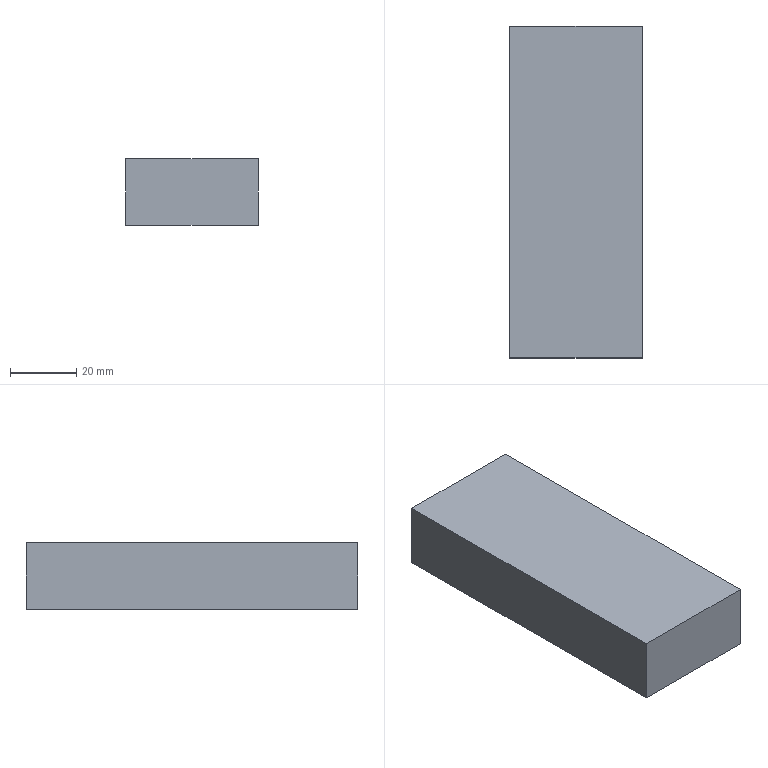Part | STEP file | 1 solid | 6 faces | box 40 x 100 x 20 mm | volume 80000 mm3 | plane 6
STEP:
#1=CARTESIAN_POINT('',(0.,0.,0.));
#2=DIRECTION('',(0.,0.,1.));
#3=DIRECTION('',(1.,0.,0.));
#4=AXIS2_PLACEMENT_3D('',#1,#2,#3);
#5=CARTESIAN_POINT('',(-20.,50.,0.));
#6=VERTEX_POINT('',#5);
#7=CARTESIAN_POINT('',(-20.,-50.,0.));
#8=VERTEX_POINT('',#7);
#9=CARTESIAN_POINT('',(-20.,50.,0.));
#10=DIRECTION('',(0.,-1.,0.));
#11=VECTOR('',#10,1.);
#12=LINE('',#9,#11);
#13=CARTESIAN_POINT('',(-20.,50.,20.));
#14=DIRECTION('',(1.,0.,0.));
#15=DIRECTION('',(0.,1.,0.));
#16=AXIS2_PLACEMENT_3D('',#13,#14,#15);
#17=PLANE('',#16);
#18=CARTESIAN_POINT('',(0.,-20.));
#19=DIRECTION('',(-1.,0.));
#20=VECTOR('',#19,1.);
#21=LINE('',#18,#20);
#22=(GEOMETRIC_REPRESENTATION_CONTEXT(2)PARAMETRIC_REPRESENTATION_CONTEXT()REPRESENTATION_CONTEXT('',''));
#23=DEFINITIONAL_REPRESENTATION('',(#21),#22);
#24=PCURVE('',#17,#23);
#25=CARTESIAN_POINT('',(0.,0.,0.));
#26=DIRECTION('',(0.,0.,-1.));
#27=DIRECTION('',(-1.,0.,0.));
#28=AXIS2_PLACEMENT_3D('',#25,#26,#27);
#29=PLANE('',#28);
#30=CARTESIAN_POINT('',(20.,50.));
#31=DIRECTION('',(0.,-1.));
#32=VECTOR('',#31,1.);
#33=LINE('',#30,#32);
#34=(GEOMETRIC_REPRESENTATION_CONTEXT(2)PARAMETRIC_REPRESENTATION_CONTEXT()REPRESENTATION_CONTEXT('',''));
#35=DEFINITIONAL_REPRESENTATION('',(#33),#34);
#36=PCURVE('',#29,#35);
#37=SURFACE_CURVE('',#12,(#24,#36),.PCURVE_S1.);
#38=EDGE_CURVE('',#6,#8,#37,.T.);
#39=ORIENTED_EDGE('',*,*,#38,.T.);
#40=CARTESIAN_POINT('',(-20.,-50.,20.));
#41=VERTEX_POINT('',#40);
#42=CARTESIAN_POINT('',(-20.,-50.,20.));
#43=DIRECTION('',(0.,0.,-1.));
#44=VECTOR('',#43,1.);
#45=LINE('',#42,#44);
#46=CARTESIAN_POINT('',(-100.,0.));
#47=DIRECTION('',(0.,-1.));
#48=VECTOR('',#47,1.);
#49=LINE('',#46,#48);
#50=(GEOMETRIC_REPRESENTATION_CONTEXT(2)PARAMETRIC_REPRESENTATION_CONTEXT()REPRESENTATION_CONTEXT('',''));
#51=DEFINITIONAL_REPRESENTATION('',(#49),#50);
#52=PCURVE('',#17,#51);
#53=CARTESIAN_POINT('',(20.,-50.,20.));
#54=DIRECTION('',(0.,1.,0.));
#55=DIRECTION('',(0.,0.,1.));
#56=AXIS2_PLACEMENT_3D('',#53,#54,#55);
#57=PLANE('',#56);
#58=CARTESIAN_POINT('',(0.,-40.));
#59=DIRECTION('',(-1.,0.));
#60=VECTOR('',#59,1.);
#61=LINE('',#58,#60);
#62=(GEOMETRIC_REPRESENTATION_CONTEXT(2)PARAMETRIC_REPRESENTATION_CONTEXT()REPRESENTATION_CONTEXT('',''));
#63=DEFINITIONAL_REPRESENTATION('',(#61),#62);
#64=PCURVE('',#57,#63);
#65=SURFACE_CURVE('',#45,(#52,#64),.PCURVE_S1.);
#66=EDGE_CURVE('',#41,#8,#65,.T.);
#67=ORIENTED_EDGE('',*,*,#66,.F.);
#68=CARTESIAN_POINT('',(-20.,50.,20.));
#69=VERTEX_POINT('',#68);
#70=CARTESIAN_POINT('',(-20.,50.,20.));
#71=DIRECTION('',(0.,-1.,0.));
#72=VECTOR('',#71,1.);
#73=LINE('',#70,#72);
#74=CARTESIAN_POINT('',(0.,0.));
#75=DIRECTION('',(-1.,0.));
#76=VECTOR('',#75,1.);
#77=LINE('',#74,#76);
#78=(GEOMETRIC_REPRESENTATION_CONTEXT(2)PARAMETRIC_REPRESENTATION_CONTEXT()REPRESENTATION_CONTEXT('',''));
#79=DEFINITIONAL_REPRESENTATION('',(#77),#78);
#80=PCURVE('',#17,#79);
#81=CARTESIAN_POINT('',(0.,0.,20.));
#82=DIRECTION('',(0.,0.,-1.));
#83=DIRECTION('',(-1.,0.,0.));
#84=AXIS2_PLACEMENT_3D('',#81,#82,#83);
#85=PLANE('',#84);
#86=CARTESIAN_POINT('',(20.,50.));
#87=DIRECTION('',(0.,-1.));
#88=VECTOR('',#87,1.);
#89=LINE('',#86,#88);
#90=(GEOMETRIC_REPRESENTATION_CONTEXT(2)PARAMETRIC_REPRESENTATION_CONTEXT()REPRESENTATION_CONTEXT('',''));
#91=DEFINITIONAL_REPRESENTATION('',(#89),#90);
#92=PCURVE('',#85,#91);
#93=SURFACE_CURVE('',#73,(#80,#92),.PCURVE_S1.);
#94=EDGE_CURVE('',#69,#41,#93,.T.);
#95=ORIENTED_EDGE('',*,*,#94,.F.);
#96=CARTESIAN_POINT('',(-20.,50.,20.));
#97=DIRECTION('',(0.,0.,-1.));
#98=VECTOR('',#97,1.);
#99=LINE('',#96,#98);
#100=CARTESIAN_POINT('',(0.,0.));
#101=DIRECTION('',(0.,-1.));
#102=VECTOR('',#101,1.);
#103=LINE('',#100,#102);
#104=(GEOMETRIC_REPRESENTATION_CONTEXT(2)PARAMETRIC_REPRESENTATION_CONTEXT()REPRESENTATION_CONTEXT('',''));
#105=DEFINITIONAL_REPRESENTATION('',(#103),#104);
#106=PCURVE('',#17,#105);
#107=CARTESIAN_POINT('',(20.,50.,20.));
#108=DIRECTION('',(0.,-1.,0.));
#109=DIRECTION('',(0.,0.,-1.));
#110=AXIS2_PLACEMENT_3D('',#107,#108,#109);
#111=PLANE('',#110);
#112=CARTESIAN_POINT('',(0.,-40.));
#113=DIRECTION('',(1.,0.));
#114=VECTOR('',#113,1.);
#115=LINE('',#112,#114);
#116=(GEOMETRIC_REPRESENTATION_CONTEXT(2)PARAMETRIC_REPRESENTATION_CONTEXT()REPRESENTATION_CONTEXT('',''));
#117=DEFINITIONAL_REPRESENTATION('',(#115),#116);
#118=PCURVE('',#111,#117);
#119=SURFACE_CURVE('',#99,(#106,#118),.PCURVE_S1.);
#120=EDGE_CURVE('',#69,#6,#119,.T.);
#121=ORIENTED_EDGE('',*,*,#120,.T.);
#122=EDGE_LOOP('',(#39,#67,#95,#121));
#123=FACE_BOUND('',#122,.T.);
#124=ADVANCED_FACE('',(#123),#17,.F.);
#125=CARTESIAN_POINT('',(20.,-50.,0.));
#126=VERTEX_POINT('',#125);
#127=CARTESIAN_POINT('',(20.,-50.,0.));
#128=DIRECTION('',(1.,0.,0.));
#129=VECTOR('',#128,1.);
#130=LINE('',#127,#129);
#131=CARTESIAN_POINT('',(-20.,0.));
#132=DIRECTION('',(0.,1.));
#133=VECTOR('',#132,1.);
#134=LINE('',#131,#133);
#135=(GEOMETRIC_REPRESENTATION_CONTEXT(2)PARAMETRIC_REPRESENTATION_CONTEXT()REPRESENTATION_CONTEXT('',''));
#136=DEFINITIONAL_REPRESENTATION('',(#134),#135);
#137=PCURVE('',#57,#136);
#138=CARTESIAN_POINT('',(-20.,-50.));
#139=DIRECTION('',(-1.,0.));
#140=VECTOR('',#139,1.);
#141=LINE('',#138,#140);
#142=(GEOMETRIC_REPRESENTATION_CONTEXT(2)PARAMETRIC_REPRESENTATION_CONTEXT()REPRESENTATION_CONTEXT('',''));
#143=DEFINITIONAL_REPRESENTATION('',(#141),#142);
#144=PCURVE('',#29,#143);
#145=SURFACE_CURVE('',#130,(#137,#144),.PCURVE_S1.);
#146=EDGE_CURVE('',#8,#126,#145,.T.);
#147=ORIENTED_EDGE('',*,*,#146,.T.);
#148=CARTESIAN_POINT('',(20.,-50.,20.));
#149=VERTEX_POINT('',#148);
#150=CARTESIAN_POINT('',(20.,-50.,20.));
#151=DIRECTION('',(0.,0.,-1.));
#152=VECTOR('',#151,1.);
#153=LINE('',#150,#152);
#154=CARTESIAN_POINT('',(0.,0.));
#155=DIRECTION('',(-1.,0.));
#156=VECTOR('',#155,1.);
#157=LINE('',#154,#156);
#158=(GEOMETRIC_REPRESENTATION_CONTEXT(2)PARAMETRIC_REPRESENTATION_CONTEXT()REPRESENTATION_CONTEXT('',''));
#159=DEFINITIONAL_REPRESENTATION('',(#157),#158);
#160=PCURVE('',#57,#159);
#161=CARTESIAN_POINT('',(20.,50.,20.));
#162=DIRECTION('',(-1.,0.,0.));
#163=DIRECTION('',(0.,-1.,0.));
#164=AXIS2_PLACEMENT_3D('',#161,#162,#163);
#165=PLANE('',#164);
#166=CARTESIAN_POINT('',(100.,0.));
#167=DIRECTION('',(0.,-1.));
#168=VECTOR('',#167,1.);
#169=LINE('',#166,#168);
#170=(GEOMETRIC_REPRESENTATION_CONTEXT(2)PARAMETRIC_REPRESENTATION_CONTEXT()REPRESENTATION_CONTEXT('',''));
#171=DEFINITIONAL_REPRESENTATION('',(#169),#170);
#172=PCURVE('',#165,#171);
#173=SURFACE_CURVE('',#153,(#160,#172),.PCURVE_S1.);
#174=EDGE_CURVE('',#149,#126,#173,.T.);
#175=ORIENTED_EDGE('',*,*,#174,.F.);
#176=CARTESIAN_POINT('',(20.,-50.,20.));
#177=DIRECTION('',(1.,0.,0.));
#178=VECTOR('',#177,1.);
#179=LINE('',#176,#178);
#180=CARTESIAN_POINT('',(0.,0.));
#181=DIRECTION('',(0.,1.));
#182=VECTOR('',#181,1.);
#183=LINE('',#180,#182);
#184=(GEOMETRIC_REPRESENTATION_CONTEXT(2)PARAMETRIC_REPRESENTATION_CONTEXT()REPRESENTATION_CONTEXT('',''));
#185=DEFINITIONAL_REPRESENTATION('',(#183),#184);
#186=PCURVE('',#57,#185);
#187=CARTESIAN_POINT('',(-20.,-50.));
#188=DIRECTION('',(-1.,0.));
#189=VECTOR('',#188,1.);
#190=LINE('',#187,#189);
#191=(GEOMETRIC_REPRESENTATION_CONTEXT(2)PARAMETRIC_REPRESENTATION_CONTEXT()REPRESENTATION_CONTEXT('',''));
#192=DEFINITIONAL_REPRESENTATION('',(#190),#191);
#193=PCURVE('',#85,#192);
#194=SURFACE_CURVE('',#179,(#186,#193),.PCURVE_S1.);
#195=EDGE_CURVE('',#41,#149,#194,.T.);
#196=ORIENTED_EDGE('',*,*,#195,.F.);
#197=ORIENTED_EDGE('',*,*,#66,.T.);
#198=EDGE_LOOP('',(#147,#175,#196,#197));
#199=FACE_BOUND('',#198,.T.);
#200=ADVANCED_FACE('',(#199),#57,.F.);
#201=CARTESIAN_POINT('',(20.,50.,0.));
#202=VERTEX_POINT('',#201);
#203=CARTESIAN_POINT('',(20.,50.,0.));
#204=DIRECTION('',(0.,1.,0.));
#205=VECTOR('',#204,1.);
#206=LINE('',#203,#205);
#207=CARTESIAN_POINT('',(0.,-20.));
#208=DIRECTION('',(-1.,0.));
#209=VECTOR('',#208,1.);
#210=LINE('',#207,#209);
#211=(GEOMETRIC_REPRESENTATION_CONTEXT(2)PARAMETRIC_REPRESENTATION_CONTEXT()REPRESENTATION_CONTEXT('',''));
#212=DEFINITIONAL_REPRESENTATION('',(#210),#211);
#213=PCURVE('',#165,#212);
#214=CARTESIAN_POINT('',(-20.,50.));
#215=DIRECTION('',(0.,1.));
#216=VECTOR('',#215,1.);
#217=LINE('',#214,#216);
#218=(GEOMETRIC_REPRESENTATION_CONTEXT(2)PARAMETRIC_REPRESENTATION_CONTEXT()REPRESENTATION_CONTEXT('',''));
#219=DEFINITIONAL_REPRESENTATION('',(#217),#218);
#220=PCURVE('',#29,#219);
#221=SURFACE_CURVE('',#206,(#213,#220),.PCURVE_S1.);
#222=EDGE_CURVE('',#126,#202,#221,.T.);
#223=ORIENTED_EDGE('',*,*,#222,.T.);
#224=CARTESIAN_POINT('',(20.,50.,20.));
#225=VERTEX_POINT('',#224);
#226=CARTESIAN_POINT('',(20.,50.,20.));
#227=DIRECTION('',(0.,0.,-1.));
#228=VECTOR('',#227,1.);
#229=LINE('',#226,#228);
#230=CARTESIAN_POINT('',(0.,0.));
#231=DIRECTION('',(0.,-1.));
#232=VECTOR('',#231,1.);
#233=LINE('',#230,#232);
#234=(GEOMETRIC_REPRESENTATION_CONTEXT(2)PARAMETRIC_REPRESENTATION_CONTEXT()REPRESENTATION_CONTEXT('',''));
#235=DEFINITIONAL_REPRESENTATION('',(#233),#234);
#236=PCURVE('',#165,#235);
#237=CARTESIAN_POINT('',(0.,0.));
#238=DIRECTION('',(1.,0.));
#239=VECTOR('',#238,1.);
#240=LINE('',#237,#239);
#241=(GEOMETRIC_REPRESENTATION_CONTEXT(2)PARAMETRIC_REPRESENTATION_CONTEXT()REPRESENTATION_CONTEXT('',''));
#242=DEFINITIONAL_REPRESENTATION('',(#240),#241);
#243=PCURVE('',#111,#242);
#244=SURFACE_CURVE('',#229,(#236,#243),.PCURVE_S1.);
#245=EDGE_CURVE('',#225,#202,#244,.T.);
#246=ORIENTED_EDGE('',*,*,#245,.F.);
#247=CARTESIAN_POINT('',(20.,50.,20.));
#248=DIRECTION('',(0.,1.,0.));
#249=VECTOR('',#248,1.);
#250=LINE('',#247,#249);
#251=CARTESIAN_POINT('',(0.,0.));
#252=DIRECTION('',(-1.,0.));
#253=VECTOR('',#252,1.);
#254=LINE('',#251,#253);
#255=(GEOMETRIC_REPRESENTATION_CONTEXT(2)PARAMETRIC_REPRESENTATION_CONTEXT()REPRESENTATION_CONTEXT('',''));
#256=DEFINITIONAL_REPRESENTATION('',(#254),#255);
#257=PCURVE('',#165,#256);
#258=CARTESIAN_POINT('',(-20.,50.));
#259=DIRECTION('',(0.,1.));
#260=VECTOR('',#259,1.);
#261=LINE('',#258,#260);
#262=(GEOMETRIC_REPRESENTATION_CONTEXT(2)PARAMETRIC_REPRESENTATION_CONTEXT()REPRESENTATION_CONTEXT('',''));
#263=DEFINITIONAL_REPRESENTATION('',(#261),#262);
#264=PCURVE('',#85,#263);
#265=SURFACE_CURVE('',#250,(#257,#264),.PCURVE_S1.);
#266=EDGE_CURVE('',#149,#225,#265,.T.);
#267=ORIENTED_EDGE('',*,*,#266,.F.);
#268=ORIENTED_EDGE('',*,*,#174,.T.);
#269=EDGE_LOOP('',(#223,#246,#267,#268));
#270=FACE_BOUND('',#269,.T.);
#271=ADVANCED_FACE('',(#270),#165,.F.);
#272=CARTESIAN_POINT('',(20.,50.,0.));
#273=DIRECTION('',(-1.,0.,0.));
#274=VECTOR('',#273,1.);
#275=LINE('',#272,#274);
#276=CARTESIAN_POINT('',(20.,0.));
#277=DIRECTION('',(0.,-1.));
#278=VECTOR('',#277,1.);
#279=LINE('',#276,#278);
#280=(GEOMETRIC_REPRESENTATION_CONTEXT(2)PARAMETRIC_REPRESENTATION_CONTEXT()REPRESENTATION_CONTEXT('',''));
#281=DEFINITIONAL_REPRESENTATION('',(#279),#280);
#282=PCURVE('',#111,#281);
#283=CARTESIAN_POINT('',(-20.,50.));
#284=DIRECTION('',(1.,0.));
#285=VECTOR('',#284,1.);
#286=LINE('',#283,#285);
#287=(GEOMETRIC_REPRESENTATION_CONTEXT(2)PARAMETRIC_REPRESENTATION_CONTEXT()REPRESENTATION_CONTEXT('',''));
#288=DEFINITIONAL_REPRESENTATION('',(#286),#287);
#289=PCURVE('',#29,#288);
#290=SURFACE_CURVE('',#275,(#282,#289),.PCURVE_S1.);
#291=EDGE_CURVE('',#202,#6,#290,.T.);
#292=ORIENTED_EDGE('',*,*,#291,.T.);
#293=ORIENTED_EDGE('',*,*,#120,.F.);
#294=CARTESIAN_POINT('',(20.,50.,20.));
#295=DIRECTION('',(-1.,0.,0.));
#296=VECTOR('',#295,1.);
#297=LINE('',#294,#296);
#298=CARTESIAN_POINT('',(0.,0.));
#299=DIRECTION('',(0.,-1.));
#300=VECTOR('',#299,1.);
#301=LINE('',#298,#300);
#302=(GEOMETRIC_REPRESENTATION_CONTEXT(2)PARAMETRIC_REPRESENTATION_CONTEXT()REPRESENTATION_CONTEXT('',''));
#303=DEFINITIONAL_REPRESENTATION('',(#301),#302);
#304=PCURVE('',#111,#303);
#305=CARTESIAN_POINT('',(-20.,50.));
#306=DIRECTION('',(1.,0.));
#307=VECTOR('',#306,1.);
#308=LINE('',#305,#307);
#309=(GEOMETRIC_REPRESENTATION_CONTEXT(2)PARAMETRIC_REPRESENTATION_CONTEXT()REPRESENTATION_CONTEXT('',''));
#310=DEFINITIONAL_REPRESENTATION('',(#308),#309);
#311=PCURVE('',#85,#310);
#312=SURFACE_CURVE('',#297,(#304,#311),.PCURVE_S1.);
#313=EDGE_CURVE('',#225,#69,#312,.T.);
#314=ORIENTED_EDGE('',*,*,#313,.F.);
#315=ORIENTED_EDGE('',*,*,#245,.T.);
#316=EDGE_LOOP('',(#292,#293,#314,#315));
#317=FACE_BOUND('',#316,.T.);
#318=ADVANCED_FACE('',(#317),#111,.F.);
#319=ORIENTED_EDGE('',*,*,#94,.T.);
#320=ORIENTED_EDGE('',*,*,#195,.T.);
#321=ORIENTED_EDGE('',*,*,#266,.T.);
#322=ORIENTED_EDGE('',*,*,#313,.T.);
#323=EDGE_LOOP('',(#319,#320,#321,#322));
#324=FACE_BOUND('',#323,.T.);
#325=ADVANCED_FACE('',(#324),#85,.F.);
#326=ORIENTED_EDGE('',*,*,#38,.F.);
#327=ORIENTED_EDGE('',*,*,#291,.F.);
#328=ORIENTED_EDGE('',*,*,#222,.F.);
#329=ORIENTED_EDGE('',*,*,#146,.F.);
#330=EDGE_LOOP('',(#326,#327,#328,#329));
#331=FACE_BOUND('',#330,.T.);
#332=ADVANCED_FACE('',(#331),#29,.T.);
#333=CLOSED_SHELL('',(#124,#200,#271,#318,#325,#332));
#334=MANIFOLD_SOLID_BREP('',#333);
#335=(LENGTH_UNIT()NAMED_UNIT(*)SI_UNIT(.MILLI.,.METRE.));
#336=UNCERTAINTY_MEASURE_WITH_UNIT(LENGTH_MEASURE(0.0000001),#335,'','');
#337=(NAMED_UNIT(*)PLANE_ANGLE_UNIT()SI_UNIT($,.RADIAN.));
#338=(NAMED_UNIT(*)SI_UNIT($,.STERADIAN.)SOLID_ANGLE_UNIT());
#339=(GEOMETRIC_REPRESENTATION_CONTEXT(3)GLOBAL_UNCERTAINTY_ASSIGNED_CONTEXT((#336))GLOBAL_UNIT_ASSIGNED_CONTEXT((#335,#337,#338))REPRESENTATION_CONTEXT('',''));
#340=ADVANCED_BREP_SHAPE_REPRESENTATION('',(#4,#334),#339);